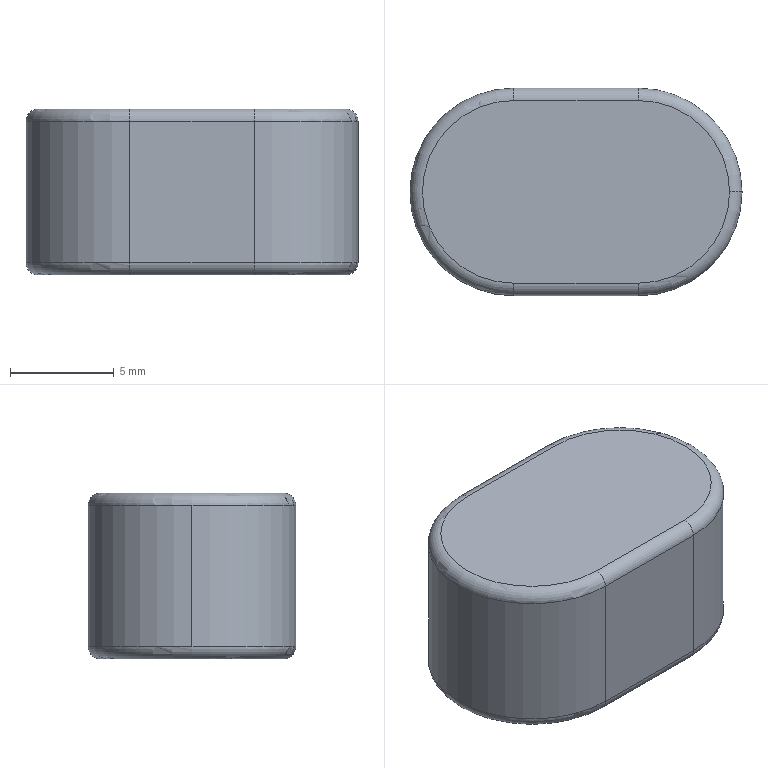Part | SolidWorks | features Extrusion 1, Fillet 1 | 1 solid | 17 faces | box 16 x 10 x 8 mm | volume 1102 mm3 | cylinder 7 | torus 6 | plane 4 | commonest cylinder face diameters 1.2 x4 10 x3
STEP:
#1=CARTESIAN_POINT('',(7.4,0.,0.));
#2=VERTEX_POINT('',#1);
#3=CARTESIAN_POINT('',(3.,-4.4,0.));
#4=VERTEX_POINT('',#3);
#5=CARTESIAN_POINT('',(3.,0.,0.));
#6=DIRECTION('',(0.,0.,-1.));
#7=DIRECTION('',(1.,0.,0.));
#8=AXIS2_PLACEMENT_3D('',#5,#6,#7);
#9=CIRCLE('',#8,4.4);
#10=EDGE_CURVE('',#2,#4,#9,.T.);
#11=ORIENTED_EDGE('',*,*,#10,.F.);
#12=CARTESIAN_POINT('',(8.,0.,0.6));
#13=VERTEX_POINT('',#12);
#14=CARTESIAN_POINT('',(7.4,0.,0.6));
#15=DIRECTION('',(0.,-1.,0.));
#16=DIRECTION('',(0.,0.,-1.));
#17=AXIS2_PLACEMENT_3D('',#14,#15,#16);
#18=CIRCLE('',#17,0.6);
#19=EDGE_CURVE('',#2,#13,#18,.T.);
#20=ORIENTED_EDGE('',*,*,#19,.T.);
#21=CARTESIAN_POINT('',(3.,-5.,0.6));
#22=VERTEX_POINT('',#21);
#23=CARTESIAN_POINT('',(3.,0.,0.6));
#24=DIRECTION('',(0.,0.,1.));
#25=DIRECTION('',(1.,0.,0.));
#26=AXIS2_PLACEMENT_3D('',#23,#24,#25);
#27=CIRCLE('',#26,5.);
#28=EDGE_CURVE('',#22,#13,#27,.T.);
#29=ORIENTED_EDGE('',*,*,#28,.F.);
#30=CARTESIAN_POINT('',(3.,-4.4,0.6));
#31=DIRECTION('',(1.,0.,0.));
#32=DIRECTION('',(0.,0.,-1.));
#33=AXIS2_PLACEMENT_3D('',#30,#31,#32);
#34=CIRCLE('',#33,0.6);
#35=EDGE_CURVE('',#22,#4,#34,.T.);
#36=ORIENTED_EDGE('',*,*,#35,.T.);
#37=EDGE_LOOP('',(#11,#20,#29,#36));
#38=FACE_OUTER_BOUND('',#37,.T.);
#39=CARTESIAN_POINT('',(3.,0.,0.6));
#40=DIRECTION('',(0.,0.,1.));
#41=DIRECTION('',(1.,0.,0.));
#42=AXIS2_PLACEMENT_3D('',#39,#40,#41);
#43=TOROIDAL_SURFACE('',#42,4.4,0.6);
#44=ADVANCED_FACE('',(#38),#43,.T.);
#45=CARTESIAN_POINT('',(8.,0.,7.4));
#46=VERTEX_POINT('',#45);
#47=CARTESIAN_POINT('',(3.,-5.,7.4));
#48=VERTEX_POINT('',#47);
#49=CARTESIAN_POINT('',(3.,0.,7.4));
#50=DIRECTION('',(0.,0.,-1.));
#51=DIRECTION('',(1.,0.,0.));
#52=AXIS2_PLACEMENT_3D('',#49,#50,#51);
#53=CIRCLE('',#52,5.);
#54=EDGE_CURVE('',#46,#48,#53,.T.);
#55=ORIENTED_EDGE('',*,*,#54,.F.);
#56=CARTESIAN_POINT('',(7.4,0.,8.));
#57=VERTEX_POINT('',#56);
#58=CARTESIAN_POINT('',(7.4,0.,7.4));
#59=DIRECTION('',(0.,-1.,0.));
#60=DIRECTION('',(0.,0.,-1.));
#61=AXIS2_PLACEMENT_3D('',#58,#59,#60);
#62=CIRCLE('',#61,0.6);
#63=EDGE_CURVE('',#46,#57,#62,.T.);
#64=ORIENTED_EDGE('',*,*,#63,.T.);
#65=CARTESIAN_POINT('',(3.,-4.4,8.));
#66=VERTEX_POINT('',#65);
#67=CARTESIAN_POINT('',(3.,0.,8.));
#68=DIRECTION('',(0.,0.,1.));
#69=DIRECTION('',(1.,0.,0.));
#70=AXIS2_PLACEMENT_3D('',#67,#68,#69);
#71=CIRCLE('',#70,4.4);
#72=EDGE_CURVE('',#66,#57,#71,.T.);
#73=ORIENTED_EDGE('',*,*,#72,.F.);
#74=CARTESIAN_POINT('',(3.,-4.4,7.4));
#75=DIRECTION('',(1.,0.,0.));
#76=DIRECTION('',(0.,0.,-1.));
#77=AXIS2_PLACEMENT_3D('',#74,#75,#76);
#78=CIRCLE('',#77,0.6);
#79=EDGE_CURVE('',#66,#48,#78,.T.);
#80=ORIENTED_EDGE('',*,*,#79,.T.);
#81=EDGE_LOOP('',(#55,#64,#73,#80));
#82=FACE_OUTER_BOUND('',#81,.T.);
#83=CARTESIAN_POINT('',(3.,0.,7.4));
#84=DIRECTION('',(0.,0.,1.));
#85=DIRECTION('',(1.,0.,0.));
#86=AXIS2_PLACEMENT_3D('',#83,#84,#85);
#87=TOROIDAL_SURFACE('',#86,4.4,0.6);
#88=ADVANCED_FACE('',(#82),#87,.T.);
#89=CARTESIAN_POINT('',(-3.,-5.,7.4));
#90=VERTEX_POINT('',#89);
#91=CARTESIAN_POINT('',(-8.,0.,7.4));
#92=VERTEX_POINT('',#91);
#93=CARTESIAN_POINT('',(-3.,0.,7.4));
#94=DIRECTION('',(0.,0.,-1.));
#95=DIRECTION('',(1.,0.,0.));
#96=AXIS2_PLACEMENT_3D('',#93,#94,#95);
#97=CIRCLE('',#96,5.);
#98=EDGE_CURVE('',#90,#92,#97,.T.);
#99=ORIENTED_EDGE('',*,*,#98,.T.);
#100=CARTESIAN_POINT('',(-8.,0.,0.6));
#101=VERTEX_POINT('',#100);
#102=CARTESIAN_POINT('',(-8.,0.,8.));
#103=DIRECTION('',(0.,0.,-1.));
#104=VECTOR('',#103,1000.);
#105=LINE('',#102,#104);
#106=EDGE_CURVE('',#92,#101,#105,.T.);
#107=ORIENTED_EDGE('',*,*,#106,.T.);
#108=CARTESIAN_POINT('',(-3.,-5.,0.6));
#109=VERTEX_POINT('',#108);
#110=CARTESIAN_POINT('',(-3.,0.,0.6));
#111=DIRECTION('',(0.,0.,1.));
#112=DIRECTION('',(1.,0.,0.));
#113=AXIS2_PLACEMENT_3D('',#110,#111,#112);
#114=CIRCLE('',#113,5.);
#115=EDGE_CURVE('',#101,#109,#114,.T.);
#116=ORIENTED_EDGE('',*,*,#115,.T.);
#117=CARTESIAN_POINT('',(-3.,-5.,8.));
#118=DIRECTION('',(0.,0.,-1.));
#119=VECTOR('',#118,1000.);
#120=LINE('',#117,#119);
#121=EDGE_CURVE('',#90,#109,#120,.T.);
#122=ORIENTED_EDGE('',*,*,#121,.F.);
#123=EDGE_LOOP('',(#99,#107,#116,#122));
#124=FACE_OUTER_BOUND('',#123,.T.);
#125=CARTESIAN_POINT('',(-3.,0.,8.));
#126=DIRECTION('',(0.,0.,-1.));
#127=DIRECTION('',(-1.,0.,0.));
#128=AXIS2_PLACEMENT_3D('',#125,#126,#127);
#129=CYLINDRICAL_SURFACE('',#128,5.);
#130=ADVANCED_FACE('',(#124),#129,.T.);
#131=ORIENTED_EDGE('',*,*,#106,.F.);
#132=CARTESIAN_POINT('',(-3.,5.,7.4));
#133=VERTEX_POINT('',#132);
#134=CARTESIAN_POINT('',(-3.,0.,7.4));
#135=DIRECTION('',(0.,0.,-1.));
#136=DIRECTION('',(1.,0.,0.));
#137=AXIS2_PLACEMENT_3D('',#134,#135,#136);
#138=CIRCLE('',#137,5.);
#139=EDGE_CURVE('',#92,#133,#138,.T.);
#140=ORIENTED_EDGE('',*,*,#139,.T.);
#141=CARTESIAN_POINT('',(-3.,5.,0.6));
#142=VERTEX_POINT('',#141);
#143=CARTESIAN_POINT('',(-3.,5.,8.));
#144=DIRECTION('',(0.,0.,-1.));
#145=VECTOR('',#144,1000.);
#146=LINE('',#143,#145);
#147=EDGE_CURVE('',#133,#142,#146,.T.);
#148=ORIENTED_EDGE('',*,*,#147,.T.);
#149=CARTESIAN_POINT('',(-3.,0.,0.6));
#150=DIRECTION('',(0.,0.,1.));
#151=DIRECTION('',(1.,0.,0.));
#152=AXIS2_PLACEMENT_3D('',#149,#150,#151);
#153=CIRCLE('',#152,5.);
#154=EDGE_CURVE('',#142,#101,#153,.T.);
#155=ORIENTED_EDGE('',*,*,#154,.T.);
#156=EDGE_LOOP('',(#131,#140,#148,#155));
#157=FACE_OUTER_BOUND('',#156,.T.);
#158=CARTESIAN_POINT('',(-3.,0.,8.));
#159=DIRECTION('',(0.,0.,-1.));
#160=DIRECTION('',(-1.,0.,0.));
#161=AXIS2_PLACEMENT_3D('',#158,#159,#160);
#162=CYLINDRICAL_SURFACE('',#161,5.);
#163=ADVANCED_FACE('',(#157),#162,.T.);
#164=CARTESIAN_POINT('',(3.,-5.,8.));
#165=DIRECTION('',(0.,0.,-1.));
#166=VECTOR('',#165,1000.);
#167=LINE('',#164,#166);
#168=EDGE_CURVE('',#48,#22,#167,.T.);
#169=ORIENTED_EDGE('',*,*,#168,.F.);
#170=CARTESIAN_POINT('',(-3.,-5.,7.4));
#171=DIRECTION('',(-1.,0.,0.));
#172=VECTOR('',#171,1000.);
#173=LINE('',#170,#172);
#174=EDGE_CURVE('',#48,#90,#173,.T.);
#175=ORIENTED_EDGE('',*,*,#174,.T.);
#176=ORIENTED_EDGE('',*,*,#121,.T.);
#177=CARTESIAN_POINT('',(-3.,-5.,0.6));
#178=DIRECTION('',(1.,0.,0.));
#179=VECTOR('',#178,1000.);
#180=LINE('',#177,#179);
#181=EDGE_CURVE('',#109,#22,#180,.T.);
#182=ORIENTED_EDGE('',*,*,#181,.T.);
#183=EDGE_LOOP('',(#169,#175,#176,#182));
#184=FACE_OUTER_BOUND('',#183,.T.);
#185=CARTESIAN_POINT('',(-3.,-5.,8.));
#186=DIRECTION('',(0.,1.,0.));
#187=DIRECTION('',(-1.,0.,0.));
#188=AXIS2_PLACEMENT_3D('',#185,#186,#187);
#189=PLANE('',#188);
#190=ADVANCED_FACE('',(#184),#189,.F.);
#191=CARTESIAN_POINT('',(3.,5.,7.4));
#192=VERTEX_POINT('',#191);
#193=CARTESIAN_POINT('',(3.,5.,0.6));
#194=VERTEX_POINT('',#193);
#195=CARTESIAN_POINT('',(3.,5.,8.));
#196=DIRECTION('',(0.,0.,-1.));
#197=VECTOR('',#196,1000.);
#198=LINE('',#195,#197);
#199=EDGE_CURVE('',#192,#194,#198,.T.);
#200=ORIENTED_EDGE('',*,*,#199,.F.);
#201=CARTESIAN_POINT('',(3.,0.,7.4));
#202=DIRECTION('',(0.,0.,-1.));
#203=DIRECTION('',(1.,0.,0.));
#204=AXIS2_PLACEMENT_3D('',#201,#202,#203);
#205=CIRCLE('',#204,5.);
#206=EDGE_CURVE('',#192,#46,#205,.T.);
#207=ORIENTED_EDGE('',*,*,#206,.T.);
#208=ORIENTED_EDGE('',*,*,#54,.T.);
#209=ORIENTED_EDGE('',*,*,#168,.T.);
#210=ORIENTED_EDGE('',*,*,#28,.T.);
#211=CARTESIAN_POINT('',(3.,0.,0.6));
#212=DIRECTION('',(0.,0.,1.));
#213=DIRECTION('',(1.,0.,0.));
#214=AXIS2_PLACEMENT_3D('',#211,#212,#213);
#215=CIRCLE('',#214,5.);
#216=EDGE_CURVE('',#13,#194,#215,.T.);
#217=ORIENTED_EDGE('',*,*,#216,.T.);
#218=EDGE_LOOP('',(#200,#207,#208,#209,#210,#217));
#219=FACE_OUTER_BOUND('',#218,.T.);
#220=CARTESIAN_POINT('',(3.,0.,8.));
#221=DIRECTION('',(0.,0.,-1.));
#222=DIRECTION('',(-1.,0.,0.));
#223=AXIS2_PLACEMENT_3D('',#220,#221,#222);
#224=CYLINDRICAL_SURFACE('',#223,5.);
#225=ADVANCED_FACE('',(#219),#224,.T.);
#226=ORIENTED_EDGE('',*,*,#147,.F.);
#227=CARTESIAN_POINT('',(3.,5.,7.4));
#228=DIRECTION('',(1.,0.,0.));
#229=VECTOR('',#228,1000.);
#230=LINE('',#227,#229);
#231=EDGE_CURVE('',#133,#192,#230,.T.);
#232=ORIENTED_EDGE('',*,*,#231,.T.);
#233=ORIENTED_EDGE('',*,*,#199,.T.);
#234=CARTESIAN_POINT('',(-3.,5.,0.6));
#235=DIRECTION('',(-1.,0.,0.));
#236=VECTOR('',#235,1000.);
#237=LINE('',#234,#236);
#238=EDGE_CURVE('',#194,#142,#237,.T.);
#239=ORIENTED_EDGE('',*,*,#238,.T.);
#240=EDGE_LOOP('',(#226,#232,#233,#239));
#241=FACE_OUTER_BOUND('',#240,.T.);
#242=CARTESIAN_POINT('',(-3.,5.,8.));
#243=DIRECTION('',(0.,-1.,0.));
#244=DIRECTION('',(1.,0.,0.));
#245=AXIS2_PLACEMENT_3D('',#242,#243,#244);
#246=PLANE('',#245);
#247=ADVANCED_FACE('',(#241),#246,.F.);
#248=CARTESIAN_POINT('',(-3.,-4.4,8.));
#249=VERTEX_POINT('',#248);
#250=CARTESIAN_POINT('',(3.,-4.4,8.));
#251=DIRECTION('',(1.,0.,0.));
#252=VECTOR('',#251,1000.);
#253=LINE('',#250,#252);
#254=EDGE_CURVE('',#249,#66,#253,.T.);
#255=ORIENTED_EDGE('',*,*,#254,.T.);
#256=ORIENTED_EDGE('',*,*,#72,.T.);
#257=CARTESIAN_POINT('',(3.,4.4,8.));
#258=VERTEX_POINT('',#257);
#259=CARTESIAN_POINT('',(3.,0.,8.));
#260=DIRECTION('',(0.,0.,1.));
#261=DIRECTION('',(1.,0.,0.));
#262=AXIS2_PLACEMENT_3D('',#259,#260,#261);
#263=CIRCLE('',#262,4.4);
#264=EDGE_CURVE('',#57,#258,#263,.T.);
#265=ORIENTED_EDGE('',*,*,#264,.T.);
#266=CARTESIAN_POINT('',(-3.,4.4,8.));
#267=VERTEX_POINT('',#266);
#268=CARTESIAN_POINT('',(-3.,4.4,8.));
#269=DIRECTION('',(-1.,0.,0.));
#270=VECTOR('',#269,1000.);
#271=LINE('',#268,#270);
#272=EDGE_CURVE('',#258,#267,#271,.T.);
#273=ORIENTED_EDGE('',*,*,#272,.T.);
#274=CARTESIAN_POINT('',(-3.,0.,8.));
#275=DIRECTION('',(0.,0.,1.));
#276=DIRECTION('',(1.,0.,0.));
#277=AXIS2_PLACEMENT_3D('',#274,#275,#276);
#278=CIRCLE('',#277,4.4);
#279=EDGE_CURVE('',#267,#249,#278,.T.);
#280=ORIENTED_EDGE('',*,*,#279,.T.);
#281=EDGE_LOOP('',(#255,#256,#265,#273,#280));
#282=FACE_OUTER_BOUND('',#281,.T.);
#283=CARTESIAN_POINT('',(-3.,0.,8.));
#284=DIRECTION('',(0.,0.,1.));
#285=DIRECTION('',(1.,0.,0.));
#286=AXIS2_PLACEMENT_3D('',#283,#284,#285);
#287=PLANE('',#286);
#288=ADVANCED_FACE('',(#282),#287,.T.);
#289=CARTESIAN_POINT('',(-3.,4.4,0.));
#290=VERTEX_POINT('',#289);
#291=CARTESIAN_POINT('',(3.,4.4,0.));
#292=VERTEX_POINT('',#291);
#293=CARTESIAN_POINT('',(-3.,4.4,0.));
#294=DIRECTION('',(1.,0.,0.));
#295=VECTOR('',#294,1000.);
#296=LINE('',#293,#295);
#297=EDGE_CURVE('',#290,#292,#296,.T.);
#298=ORIENTED_EDGE('',*,*,#297,.T.);
#299=CARTESIAN_POINT('',(3.,0.,0.));
#300=DIRECTION('',(0.,0.,-1.));
#301=DIRECTION('',(1.,0.,0.));
#302=AXIS2_PLACEMENT_3D('',#299,#300,#301);
#303=CIRCLE('',#302,4.4);
#304=EDGE_CURVE('',#292,#2,#303,.T.);
#305=ORIENTED_EDGE('',*,*,#304,.T.);
#306=ORIENTED_EDGE('',*,*,#10,.T.);
#307=CARTESIAN_POINT('',(-3.,-4.4,0.));
#308=VERTEX_POINT('',#307);
#309=CARTESIAN_POINT('',(-3.,-4.4,0.));
#310=DIRECTION('',(-1.,0.,0.));
#311=VECTOR('',#310,1000.);
#312=LINE('',#309,#311);
#313=EDGE_CURVE('',#4,#308,#312,.T.);
#314=ORIENTED_EDGE('',*,*,#313,.T.);
#315=CARTESIAN_POINT('',(-3.,0.,0.));
#316=DIRECTION('',(0.,0.,-1.));
#317=DIRECTION('',(1.,0.,0.));
#318=AXIS2_PLACEMENT_3D('',#315,#316,#317);
#319=CIRCLE('',#318,4.4);
#320=EDGE_CURVE('',#308,#290,#319,.T.);
#321=ORIENTED_EDGE('',*,*,#320,.T.);
#322=EDGE_LOOP('',(#298,#305,#306,#314,#321));
#323=FACE_OUTER_BOUND('',#322,.T.);
#324=CARTESIAN_POINT('',(-3.,0.,0.));
#325=DIRECTION('',(0.,0.,1.));
#326=DIRECTION('',(1.,0.,0.));
#327=AXIS2_PLACEMENT_3D('',#324,#325,#326);
#328=PLANE('',#327);
#329=ADVANCED_FACE('',(#323),#328,.F.);
#330=CARTESIAN_POINT('',(-3.,4.4,7.4));
#331=DIRECTION('',(1.,0.,0.));
#332=DIRECTION('',(0.,0.,-1.));
#333=AXIS2_PLACEMENT_3D('',#330,#331,#332);
#334=CIRCLE('',#333,0.6);
#335=EDGE_CURVE('',#133,#267,#334,.T.);
#336=ORIENTED_EDGE('',*,*,#335,.F.);
#337=ORIENTED_EDGE('',*,*,#139,.F.);
#338=ORIENTED_EDGE('',*,*,#98,.F.);
#339=CARTESIAN_POINT('',(-3.,-4.4,7.4));
#340=DIRECTION('',(1.,0.,0.));
#341=DIRECTION('',(0.,0.,-1.));
#342=AXIS2_PLACEMENT_3D('',#339,#340,#341);
#343=CIRCLE('',#342,0.6);
#344=EDGE_CURVE('',#249,#90,#343,.T.);
#345=ORIENTED_EDGE('',*,*,#344,.F.);
#346=ORIENTED_EDGE('',*,*,#279,.F.);
#347=EDGE_LOOP('',(#336,#337,#338,#345,#346));
#348=FACE_OUTER_BOUND('',#347,.T.);
#349=CARTESIAN_POINT('',(-3.,0.,7.4));
#350=DIRECTION('',(0.,0.,1.));
#351=DIRECTION('',(1.,0.,0.));
#352=AXIS2_PLACEMENT_3D('',#349,#350,#351);
#353=TOROIDAL_SURFACE('',#352,4.4,0.6);
#354=ADVANCED_FACE('',(#348),#353,.T.);
#355=ORIENTED_EDGE('',*,*,#344,.T.);
#356=ORIENTED_EDGE('',*,*,#174,.F.);
#357=ORIENTED_EDGE('',*,*,#79,.F.);
#358=ORIENTED_EDGE('',*,*,#254,.F.);
#359=EDGE_LOOP('',(#355,#356,#357,#358));
#360=FACE_OUTER_BOUND('',#359,.T.);
#361=CARTESIAN_POINT('',(-3.,-4.4,7.4));
#362=DIRECTION('',(-1.,0.,0.));
#363=DIRECTION('',(0.,-1.,0.));
#364=AXIS2_PLACEMENT_3D('',#361,#362,#363);
#365=CYLINDRICAL_SURFACE('',#364,0.6);
#366=ADVANCED_FACE('',(#360),#365,.T.);
#367=ORIENTED_EDGE('',*,*,#335,.T.);
#368=ORIENTED_EDGE('',*,*,#272,.F.);
#369=CARTESIAN_POINT('',(3.,4.4,7.4));
#370=DIRECTION('',(1.,0.,0.));
#371=DIRECTION('',(0.,0.,-1.));
#372=AXIS2_PLACEMENT_3D('',#369,#370,#371);
#373=CIRCLE('',#372,0.6);
#374=EDGE_CURVE('',#192,#258,#373,.T.);
#375=ORIENTED_EDGE('',*,*,#374,.F.);
#376=ORIENTED_EDGE('',*,*,#231,.F.);
#377=EDGE_LOOP('',(#367,#368,#375,#376));
#378=FACE_OUTER_BOUND('',#377,.T.);
#379=CARTESIAN_POINT('',(-3.,4.4,7.4));
#380=DIRECTION('',(1.,0.,0.));
#381=DIRECTION('',(0.,1.,0.));
#382=AXIS2_PLACEMENT_3D('',#379,#380,#381);
#383=CYLINDRICAL_SURFACE('',#382,0.6);
#384=ADVANCED_FACE('',(#378),#383,.T.);
#385=ORIENTED_EDGE('',*,*,#63,.F.);
#386=ORIENTED_EDGE('',*,*,#206,.F.);
#387=ORIENTED_EDGE('',*,*,#374,.T.);
#388=ORIENTED_EDGE('',*,*,#264,.F.);
#389=EDGE_LOOP('',(#385,#386,#387,#388));
#390=FACE_OUTER_BOUND('',#389,.T.);
#391=CARTESIAN_POINT('',(3.,0.,7.4));
#392=DIRECTION('',(0.,0.,1.));
#393=DIRECTION('',(1.,0.,0.));
#394=AXIS2_PLACEMENT_3D('',#391,#392,#393);
#395=TOROIDAL_SURFACE('',#394,4.4,0.6);
#396=ADVANCED_FACE('',(#390),#395,.T.);
#397=CARTESIAN_POINT('',(-3.,4.4,0.6));
#398=DIRECTION('',(1.,0.,0.));
#399=DIRECTION('',(0.,0.,-1.));
#400=AXIS2_PLACEMENT_3D('',#397,#398,#399);
#401=CIRCLE('',#400,0.6);
#402=EDGE_CURVE('',#290,#142,#401,.T.);
#403=ORIENTED_EDGE('',*,*,#402,.F.);
#404=ORIENTED_EDGE('',*,*,#320,.F.);
#405=CARTESIAN_POINT('',(-3.,-4.4,0.6));
#406=DIRECTION('',(1.,0.,0.));
#407=DIRECTION('',(0.,0.,-1.));
#408=AXIS2_PLACEMENT_3D('',#405,#406,#407);
#409=CIRCLE('',#408,0.6);
#410=EDGE_CURVE('',#109,#308,#409,.T.);
#411=ORIENTED_EDGE('',*,*,#410,.F.);
#412=ORIENTED_EDGE('',*,*,#115,.F.);
#413=ORIENTED_EDGE('',*,*,#154,.F.);
#414=EDGE_LOOP('',(#403,#404,#411,#412,#413));
#415=FACE_OUTER_BOUND('',#414,.T.);
#416=CARTESIAN_POINT('',(-3.,0.,0.6));
#417=DIRECTION('',(0.,0.,1.));
#418=DIRECTION('',(1.,0.,0.));
#419=AXIS2_PLACEMENT_3D('',#416,#417,#418);
#420=TOROIDAL_SURFACE('',#419,4.4,0.6);
#421=ADVANCED_FACE('',(#415),#420,.T.);
#422=ORIENTED_EDGE('',*,*,#410,.T.);
#423=ORIENTED_EDGE('',*,*,#313,.F.);
#424=ORIENTED_EDGE('',*,*,#35,.F.);
#425=ORIENTED_EDGE('',*,*,#181,.F.);
#426=EDGE_LOOP('',(#422,#423,#424,#425));
#427=FACE_OUTER_BOUND('',#426,.T.);
#428=CARTESIAN_POINT('',(-3.,-4.4,0.6));
#429=DIRECTION('',(1.,0.,0.));
#430=DIRECTION('',(0.,1.,0.));
#431=AXIS2_PLACEMENT_3D('',#428,#429,#430);
#432=CYLINDRICAL_SURFACE('',#431,0.6);
#433=ADVANCED_FACE('',(#427),#432,.T.);
#434=ORIENTED_EDGE('',*,*,#402,.T.);
#435=ORIENTED_EDGE('',*,*,#238,.F.);
#436=CARTESIAN_POINT('',(3.,4.4,0.6));
#437=DIRECTION('',(1.,0.,0.));
#438=DIRECTION('',(0.,0.,-1.));
#439=AXIS2_PLACEMENT_3D('',#436,#437,#438);
#440=CIRCLE('',#439,0.6);
#441=EDGE_CURVE('',#292,#194,#440,.T.);
#442=ORIENTED_EDGE('',*,*,#441,.F.);
#443=ORIENTED_EDGE('',*,*,#297,.F.);
#444=EDGE_LOOP('',(#434,#435,#442,#443));
#445=FACE_OUTER_BOUND('',#444,.T.);
#446=CARTESIAN_POINT('',(-3.,4.4,0.6));
#447=DIRECTION('',(-1.,0.,0.));
#448=DIRECTION('',(0.,-1.,0.));
#449=AXIS2_PLACEMENT_3D('',#446,#447,#448);
#450=CYLINDRICAL_SURFACE('',#449,0.6);
#451=ADVANCED_FACE('',(#445),#450,.T.);
#452=ORIENTED_EDGE('',*,*,#19,.F.);
#453=ORIENTED_EDGE('',*,*,#304,.F.);
#454=ORIENTED_EDGE('',*,*,#441,.T.);
#455=ORIENTED_EDGE('',*,*,#216,.F.);
#456=EDGE_LOOP('',(#452,#453,#454,#455));
#457=FACE_OUTER_BOUND('',#456,.T.);
#458=CARTESIAN_POINT('',(3.,0.,0.6));
#459=DIRECTION('',(0.,0.,1.));
#460=DIRECTION('',(1.,0.,0.));
#461=AXIS2_PLACEMENT_3D('',#458,#459,#460);
#462=TOROIDAL_SURFACE('',#461,4.4,0.6);
#463=ADVANCED_FACE('',(#457),#462,.T.);
#464=CLOSED_SHELL('',(#44,#88,#130,#163,#190,#225,#247,#288,#329,#354,#366,#384,#396,#421,#433,#451,#463));
#465=MANIFOLD_SOLID_BREP('',#464);
#466=CARTESIAN_POINT('',(0.,0.,0.));
#467=DIRECTION('',(0.,0.,1.));
#468=DIRECTION('',(1.,0.,0.));
#469=AXIS2_PLACEMENT_3D('',#466,#467,#468);
#470=(LENGTH_UNIT()NAMED_UNIT(*)SI_UNIT(.MILLI.,.METRE.));
#471=UNCERTAINTY_MEASURE_WITH_UNIT(LENGTH_MEASURE(0.00001),#470,'','');
#472=(NAMED_UNIT(*)PLANE_ANGLE_UNIT()SI_UNIT($,.RADIAN.));
#473=(NAMED_UNIT(*)SI_UNIT($,.STERADIAN.)SOLID_ANGLE_UNIT());
#474=(GEOMETRIC_REPRESENTATION_CONTEXT(3)GLOBAL_UNCERTAINTY_ASSIGNED_CONTEXT((#471))GLOBAL_UNIT_ASSIGNED_CONTEXT((#470,#472,#473))REPRESENTATION_CONTEXT('',''));
#475=ADVANCED_BREP_SHAPE_REPRESENTATION('',(#465,#469),#474);